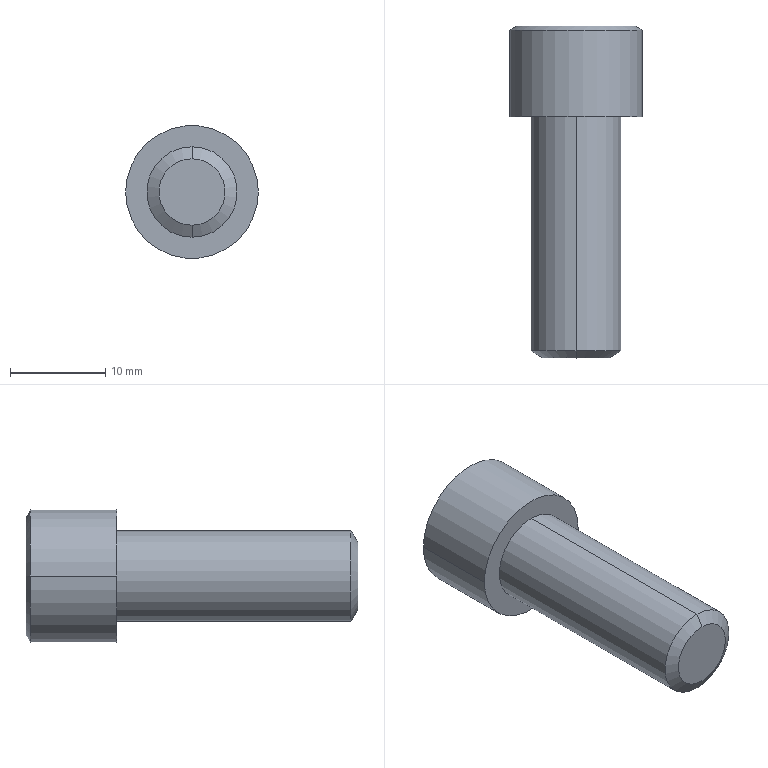Part | NX | features BREP 1 | 1 solid | 11 faces | box 13.97 x 34.925 x 13.97 mm | volume 3250 mm3 | cone 4 | cylinder 4 | plane 3 | commonest cylinder face diameters 9.525 x2 13.97 x2
STEP:
#1=CARTESIAN_POINT('',(0.,-25.4,3.493));
#2=VERTEX_POINT('',#1);
#3=CARTESIAN_POINT('',(0.,-25.4,-3.493));
#4=VERTEX_POINT('',#3);
#5=CARTESIAN_POINT('',(0.,-25.4,0.));
#6=DIRECTION('',(0.,-1.,0.));
#7=DIRECTION('',(0.,0.,1.));
#8=AXIS2_PLACEMENT_3D('',#5,#6,#7);
#9=CIRCLE('',#8,3.493);
#10=EDGE_CURVE('',#2,#4,#9,.T.);
#11=ORIENTED_EDGE('',*,*,#10,.T.);
#12=CARTESIAN_POINT('',(0.,-25.4,0.));
#13=DIRECTION('',(0.,-1.,0.));
#14=DIRECTION('',(0.,0.,-1.));
#15=AXIS2_PLACEMENT_3D('',#12,#13,#14);
#16=CIRCLE('',#15,3.493);
#17=EDGE_CURVE('',#4,#2,#16,.T.);
#18=ORIENTED_EDGE('',*,*,#17,.T.);
#19=EDGE_LOOP('',(#11,#18));
#20=FACE_BOUND('',#19,.T.);
#21=CARTESIAN_POINT('',(0.,-25.4,0.));
#22=DIRECTION('',(0.,-1.,0.));
#23=DIRECTION('',(0.,0.,-1.));
#24=AXIS2_PLACEMENT_3D('',#21,#22,#23);
#25=PLANE('',#24);
#26=ADVANCED_FACE('',(#20),#25,.T.);
#27=CARTESIAN_POINT('',(0.,-24.667,-4.763));
#28=VERTEX_POINT('',#27);
#29=CARTESIAN_POINT('',(0.,-25.4,-3.493));
#30=DIRECTION('',(0.,0.5,-0.866));
#31=VECTOR('',#30,1000.);
#32=LINE('',#29,#31);
#33=EDGE_CURVE('',#4,#28,#32,.T.);
#34=ORIENTED_EDGE('',*,*,#33,.T.);
#35=CARTESIAN_POINT('',(0.,-24.667,4.763));
#36=VERTEX_POINT('',#35);
#37=CARTESIAN_POINT('',(0.,-24.667,0.));
#38=DIRECTION('',(0.,-1.,0.));
#39=DIRECTION('',(0.,0.,-1.));
#40=AXIS2_PLACEMENT_3D('',#37,#38,#39);
#41=CIRCLE('',#40,4.763);
#42=EDGE_CURVE('',#28,#36,#41,.T.);
#43=ORIENTED_EDGE('',*,*,#42,.T.);
#44=CARTESIAN_POINT('',(0.,-25.4,3.493));
#45=DIRECTION('',(0.,0.5,0.866));
#46=VECTOR('',#45,1000.);
#47=LINE('',#44,#46);
#48=EDGE_CURVE('',#2,#36,#47,.T.);
#49=ORIENTED_EDGE('',*,*,#48,.F.);
#50=ORIENTED_EDGE('',*,*,#17,.F.);
#51=EDGE_LOOP('',(#34,#43,#49,#50));
#52=FACE_BOUND('',#51,.T.);
#53=CARTESIAN_POINT('',(0.,-25.033,0.));
#54=DIRECTION('',(0.,1.,0.));
#55=DIRECTION('',(0.,0.,1.));
#56=AXIS2_PLACEMENT_3D('',#53,#54,#55);
#57=CONICAL_SURFACE('',#56,4.128,1.047);
#58=ADVANCED_FACE('',(#52),#57,.T.);
#59=ORIENTED_EDGE('',*,*,#48,.T.);
#60=CARTESIAN_POINT('',(0.,-24.667,0.));
#61=DIRECTION('',(0.,-1.,0.));
#62=DIRECTION('',(0.,0.,1.));
#63=AXIS2_PLACEMENT_3D('',#60,#61,#62);
#64=CIRCLE('',#63,4.763);
#65=EDGE_CURVE('',#36,#28,#64,.T.);
#66=ORIENTED_EDGE('',*,*,#65,.T.);
#67=ORIENTED_EDGE('',*,*,#33,.F.);
#68=ORIENTED_EDGE('',*,*,#10,.F.);
#69=EDGE_LOOP('',(#59,#66,#67,#68));
#70=FACE_BOUND('',#69,.T.);
#71=CARTESIAN_POINT('',(0.,-25.033,0.));
#72=DIRECTION('',(0.,1.,0.));
#73=DIRECTION('',(0.,0.,1.));
#74=AXIS2_PLACEMENT_3D('',#71,#72,#73);
#75=CONICAL_SURFACE('',#74,4.128,1.047);
#76=ADVANCED_FACE('',(#70),#75,.T.);
#77=CARTESIAN_POINT('',(0.,0.,-4.763));
#78=VERTEX_POINT('',#77);
#79=CARTESIAN_POINT('',(0.,0.,-4.763));
#80=DIRECTION('',(0.,-1.,0.));
#81=VECTOR('',#80,1000.);
#82=LINE('',#79,#81);
#83=EDGE_CURVE('',#78,#28,#82,.T.);
#84=ORIENTED_EDGE('',*,*,#83,.T.);
#85=ORIENTED_EDGE('',*,*,#65,.F.);
#86=CARTESIAN_POINT('',(0.,0.,4.763));
#87=VERTEX_POINT('',#86);
#88=CARTESIAN_POINT('',(0.,0.,4.763));
#89=DIRECTION('',(0.,-1.,0.));
#90=VECTOR('',#89,1000.);
#91=LINE('',#88,#90);
#92=EDGE_CURVE('',#87,#36,#91,.T.);
#93=ORIENTED_EDGE('',*,*,#92,.F.);
#94=CARTESIAN_POINT('',(0.,0.,0.));
#95=DIRECTION('',(0.,-1.,0.));
#96=DIRECTION('',(0.,0.,1.));
#97=AXIS2_PLACEMENT_3D('',#94,#95,#96);
#98=CIRCLE('',#97,4.763);
#99=EDGE_CURVE('',#87,#78,#98,.T.);
#100=ORIENTED_EDGE('',*,*,#99,.T.);
#101=EDGE_LOOP('',(#84,#85,#93,#100));
#102=FACE_BOUND('',#101,.T.);
#103=CARTESIAN_POINT('',(0.,0.,0.));
#104=DIRECTION('',(0.,-1.,0.));
#105=DIRECTION('',(0.,0.,-1.));
#106=AXIS2_PLACEMENT_3D('',#103,#104,#105);
#107=CYLINDRICAL_SURFACE('',#106,4.763);
#108=ADVANCED_FACE('',(#102),#107,.T.);
#109=CARTESIAN_POINT('',(-6.985,0.,0.));
#110=VERTEX_POINT('',#109);
#111=CARTESIAN_POINT('',(6.985,0.,0.));
#112=VERTEX_POINT('',#111);
#113=CARTESIAN_POINT('',(0.,0.,0.));
#114=DIRECTION('',(0.,1.,0.));
#115=DIRECTION('',(-1.,0.,0.));
#116=AXIS2_PLACEMENT_3D('',#113,#114,#115);
#117=CIRCLE('',#116,6.985);
#118=EDGE_CURVE('',#110,#112,#117,.T.);
#119=ORIENTED_EDGE('',*,*,#118,.F.);
#120=CARTESIAN_POINT('',(0.,0.,0.));
#121=DIRECTION('',(0.,1.,0.));
#122=DIRECTION('',(1.,0.,0.));
#123=AXIS2_PLACEMENT_3D('',#120,#121,#122);
#124=CIRCLE('',#123,6.985);
#125=EDGE_CURVE('',#112,#110,#124,.T.);
#126=ORIENTED_EDGE('',*,*,#125,.F.);
#127=EDGE_LOOP('',(#119,#126));
#128=FACE_BOUND('',#127,.T.);
#129=ORIENTED_EDGE('',*,*,#99,.F.);
#130=CARTESIAN_POINT('',(0.,0.,0.));
#131=DIRECTION('',(0.,-1.,0.));
#132=DIRECTION('',(0.,0.,-1.));
#133=AXIS2_PLACEMENT_3D('',#130,#131,#132);
#134=CIRCLE('',#133,4.763);
#135=EDGE_CURVE('',#78,#87,#134,.T.);
#136=ORIENTED_EDGE('',*,*,#135,.F.);
#137=EDGE_LOOP('',(#129,#136));
#138=FACE_BOUND('',#137,.T.);
#139=CARTESIAN_POINT('',(0.,0.,0.));
#140=DIRECTION('',(0.,1.,0.));
#141=DIRECTION('',(1.,0.,0.));
#142=AXIS2_PLACEMENT_3D('',#139,#140,#141);
#143=PLANE('',#142);
#144=ADVANCED_FACE('',(#128,#138),#143,.F.);
#145=CARTESIAN_POINT('',(-6.985,9.085,0.));
#146=VERTEX_POINT('',#145);
#147=CARTESIAN_POINT('',(-6.985,0.,0.));
#148=DIRECTION('',(0.,1.,0.));
#149=VECTOR('',#148,1000.);
#150=LINE('',#147,#149);
#151=EDGE_CURVE('',#110,#146,#150,.T.);
#152=ORIENTED_EDGE('',*,*,#151,.T.);
#153=CARTESIAN_POINT('',(6.985,9.085,0.));
#154=VERTEX_POINT('',#153);
#155=CARTESIAN_POINT('',(0.,9.085,0.));
#156=DIRECTION('',(0.,1.,0.));
#157=DIRECTION('',(1.,0.,0.));
#158=AXIS2_PLACEMENT_3D('',#155,#156,#157);
#159=CIRCLE('',#158,6.985);
#160=EDGE_CURVE('',#154,#146,#159,.T.);
#161=ORIENTED_EDGE('',*,*,#160,.F.);
#162=CARTESIAN_POINT('',(6.985,0.,0.));
#163=DIRECTION('',(0.,1.,0.));
#164=VECTOR('',#163,1000.);
#165=LINE('',#162,#164);
#166=EDGE_CURVE('',#112,#154,#165,.T.);
#167=ORIENTED_EDGE('',*,*,#166,.F.);
#168=ORIENTED_EDGE('',*,*,#125,.T.);
#169=EDGE_LOOP('',(#152,#161,#167,#168));
#170=FACE_BOUND('',#169,.T.);
#171=CARTESIAN_POINT('',(0.,0.,0.));
#172=DIRECTION('',(0.,1.,0.));
#173=DIRECTION('',(1.,0.,0.));
#174=AXIS2_PLACEMENT_3D('',#171,#172,#173);
#175=CYLINDRICAL_SURFACE('',#174,6.985);
#176=ADVANCED_FACE('',(#170),#175,.T.);
#177=ORIENTED_EDGE('',*,*,#166,.T.);
#178=CARTESIAN_POINT('',(0.,9.085,0.));
#179=DIRECTION('',(0.,1.,0.));
#180=DIRECTION('',(-1.,0.,0.));
#181=AXIS2_PLACEMENT_3D('',#178,#179,#180);
#182=CIRCLE('',#181,6.985);
#183=EDGE_CURVE('',#146,#154,#182,.T.);
#184=ORIENTED_EDGE('',*,*,#183,.F.);
#185=ORIENTED_EDGE('',*,*,#151,.F.);
#186=ORIENTED_EDGE('',*,*,#118,.T.);
#187=EDGE_LOOP('',(#177,#184,#185,#186));
#188=FACE_BOUND('',#187,.T.);
#189=CARTESIAN_POINT('',(0.,0.,0.));
#190=DIRECTION('',(0.,1.,0.));
#191=DIRECTION('',(1.,0.,0.));
#192=AXIS2_PLACEMENT_3D('',#189,#190,#191);
#193=CYLINDRICAL_SURFACE('',#192,6.985);
#194=ADVANCED_FACE('',(#188),#193,.T.);
#195=CARTESIAN_POINT('',(-6.223,9.525,0.));
#196=VERTEX_POINT('',#195);
#197=CARTESIAN_POINT('',(-6.223,9.525,0.));
#198=DIRECTION('',(-0.866,-0.5,0.));
#199=VECTOR('',#198,1000.);
#200=LINE('',#197,#199);
#201=EDGE_CURVE('',#196,#146,#200,.T.);
#202=ORIENTED_EDGE('',*,*,#201,.T.);
#203=ORIENTED_EDGE('',*,*,#183,.T.);
#204=CARTESIAN_POINT('',(6.223,9.525,0.));
#205=VERTEX_POINT('',#204);
#206=CARTESIAN_POINT('',(6.223,9.525,0.));
#207=DIRECTION('',(0.866,-0.5,0.));
#208=VECTOR('',#207,1000.);
#209=LINE('',#206,#208);
#210=EDGE_CURVE('',#205,#154,#209,.T.);
#211=ORIENTED_EDGE('',*,*,#210,.F.);
#212=CARTESIAN_POINT('',(0.,9.525,0.));
#213=DIRECTION('',(0.,1.,0.));
#214=DIRECTION('',(-1.,0.,0.));
#215=AXIS2_PLACEMENT_3D('',#212,#213,#214);
#216=CIRCLE('',#215,6.223);
#217=EDGE_CURVE('',#196,#205,#216,.T.);
#218=ORIENTED_EDGE('',*,*,#217,.F.);
#219=EDGE_LOOP('',(#202,#203,#211,#218));
#220=FACE_BOUND('',#219,.T.);
#221=CARTESIAN_POINT('',(0.,9.305,0.));
#222=DIRECTION('',(0.,-1.,0.));
#223=DIRECTION('',(-1.,0.,0.));
#224=AXIS2_PLACEMENT_3D('',#221,#222,#223);
#225=CONICAL_SURFACE('',#224,6.604,1.047);
#226=ADVANCED_FACE('',(#220),#225,.T.);
#227=ORIENTED_EDGE('',*,*,#217,.T.);
#228=CARTESIAN_POINT('',(0.,9.525,0.));
#229=DIRECTION('',(0.,1.,0.));
#230=DIRECTION('',(1.,0.,0.));
#231=AXIS2_PLACEMENT_3D('',#228,#229,#230);
#232=CIRCLE('',#231,6.223);
#233=EDGE_CURVE('',#205,#196,#232,.T.);
#234=ORIENTED_EDGE('',*,*,#233,.T.);
#235=EDGE_LOOP('',(#227,#234));
#236=FACE_BOUND('',#235,.T.);
#237=CARTESIAN_POINT('',(0.,9.525,0.));
#238=DIRECTION('',(0.,1.,0.));
#239=DIRECTION('',(1.,0.,0.));
#240=AXIS2_PLACEMENT_3D('',#237,#238,#239);
#241=PLANE('',#240);
#242=ADVANCED_FACE('',(#236),#241,.T.);
#243=ORIENTED_EDGE('',*,*,#210,.T.);
#244=ORIENTED_EDGE('',*,*,#160,.T.);
#245=ORIENTED_EDGE('',*,*,#201,.F.);
#246=ORIENTED_EDGE('',*,*,#233,.F.);
#247=EDGE_LOOP('',(#243,#244,#245,#246));
#248=FACE_BOUND('',#247,.T.);
#249=CARTESIAN_POINT('',(0.,9.305,0.));
#250=DIRECTION('',(0.,-1.,0.));
#251=DIRECTION('',(-1.,0.,0.));
#252=AXIS2_PLACEMENT_3D('',#249,#250,#251);
#253=CONICAL_SURFACE('',#252,6.604,1.047);
#254=ADVANCED_FACE('',(#248),#253,.T.);
#255=ORIENTED_EDGE('',*,*,#92,.T.);
#256=ORIENTED_EDGE('',*,*,#42,.F.);
#257=ORIENTED_EDGE('',*,*,#83,.F.);
#258=ORIENTED_EDGE('',*,*,#135,.T.);
#259=EDGE_LOOP('',(#255,#256,#257,#258));
#260=FACE_BOUND('',#259,.T.);
#261=CARTESIAN_POINT('',(0.,0.,0.));
#262=DIRECTION('',(0.,-1.,0.));
#263=DIRECTION('',(0.,0.,-1.));
#264=AXIS2_PLACEMENT_3D('',#261,#262,#263);
#265=CYLINDRICAL_SURFACE('',#264,4.763);
#266=ADVANCED_FACE('',(#260),#265,.T.);
#267=CLOSED_SHELL('',(#26,#58,#76,#108,#144,#176,#194,#226,#242,#254,#266));
#268=MANIFOLD_SOLID_BREP('',#267);
#269=(LENGTH_UNIT()NAMED_UNIT(*)SI_UNIT(.MILLI.,.METRE.));
#270=UNCERTAINTY_MEASURE_WITH_UNIT(LENGTH_MEASURE(0.00001),#269,'','');
#271=(NAMED_UNIT(*)PLANE_ANGLE_UNIT()SI_UNIT($,.RADIAN.));
#272=(NAMED_UNIT(*)SI_UNIT($,.STERADIAN.)SOLID_ANGLE_UNIT());
#273=(GEOMETRIC_REPRESENTATION_CONTEXT(3)GLOBAL_UNCERTAINTY_ASSIGNED_CONTEXT((#270))GLOBAL_UNIT_ASSIGNED_CONTEXT((#269,#271,#272))REPRESENTATION_CONTEXT('',''));
#274=ADVANCED_BREP_SHAPE_REPRESENTATION('',(#268),#273);